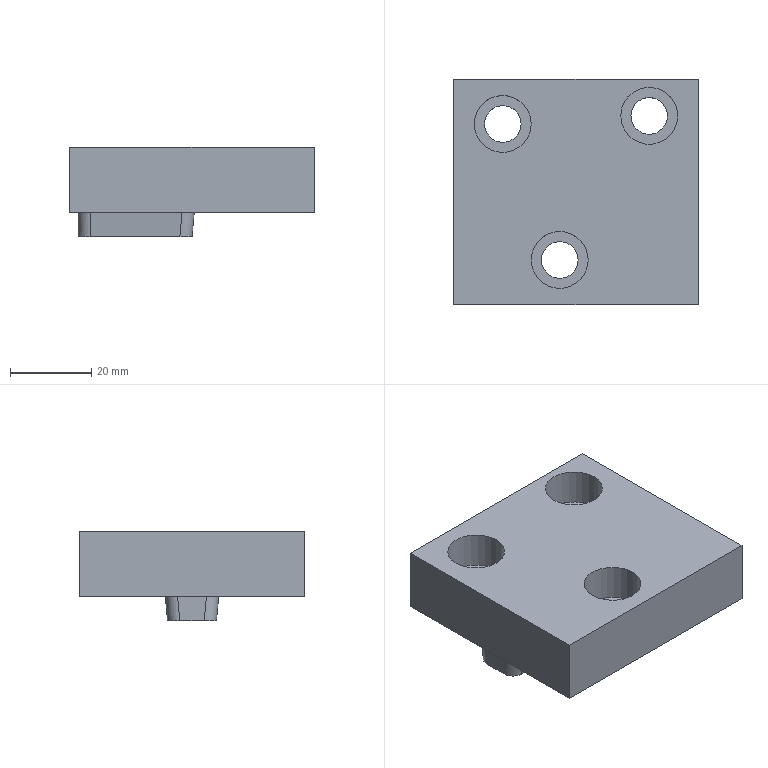Part | STEP file | solid 10 | 1 solid | 24 faces | box 60 x 55.425 x 22 mm | volume 49802 mm3 | plane 14 | cylinder 10 | commonest cylinder face diameters 6 x4 9 x3 14 x3